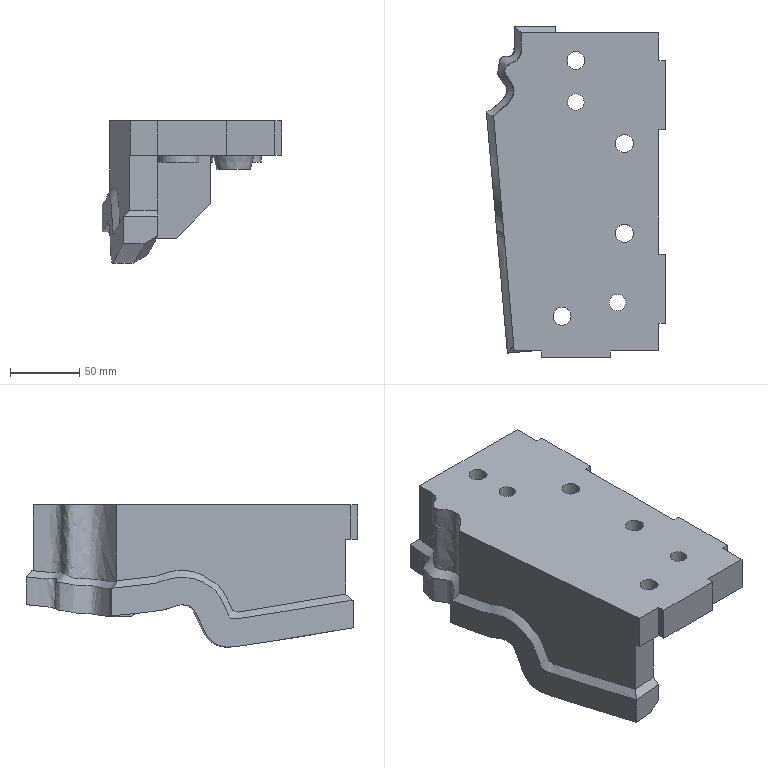Part | NX | features solid 2 | 1 solid | 63 faces | box 129.841 x 240 x 103.025 mm | volume 1046246 mm3 | plane 40 | cylinder 12 | spline 9 | cone 2 | commonest cylinder face diameters 13 x6 30 x4 12 x2